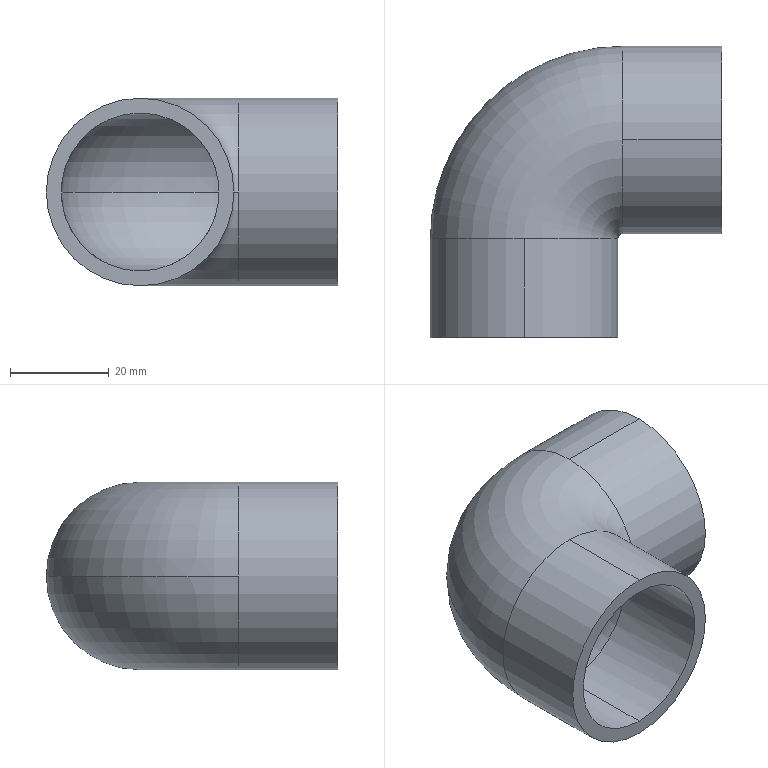Part | SolidWorks | features Sweep 1 | 1 solid | 14 faces | box 59 x 59 x 38 mm | volume 23558 mm3 | cylinder 8 | torus 4 | plane 2 | commonest cylinder face diameters 32 x4 38 x4
STEP:
#1=CARTESIAN_POINT('',(-16.,20.,0.));
#2=VERTEX_POINT('',#1);
#3=CARTESIAN_POINT('',(0.,20.,16.));
#4=VERTEX_POINT('',#3);
#5=CARTESIAN_POINT('',(0.,20.,0.));
#6=DIRECTION('',(0.,1.,0.));
#7=DIRECTION('',(0.,0.,1.));
#8=AXIS2_PLACEMENT_3D('',#5,#6,#7);
#9=CIRCLE('',#8,16.);
#10=EDGE_CURVE('',#2,#4,#9,.T.);
#11=ORIENTED_EDGE('',*,*,#10,.F.);
#12=CARTESIAN_POINT('',(20.,56.,0.));
#13=VERTEX_POINT('',#12);
#14=CARTESIAN_POINT('',(20.,20.,0.));
#15=DIRECTION('',(0.,0.,-1.));
#16=DIRECTION('',(-1.,0.,0.));
#17=AXIS2_PLACEMENT_3D('',#14,#15,#16);
#18=CIRCLE('',#17,36.);
#19=EDGE_CURVE('',#2,#13,#18,.T.);
#20=ORIENTED_EDGE('',*,*,#19,.T.);
#21=CARTESIAN_POINT('',(20.,40.,16.));
#22=VERTEX_POINT('',#21);
#23=CARTESIAN_POINT('',(20.,40.,0.));
#24=DIRECTION('',(1.,0.,0.));
#25=DIRECTION('',(0.,0.,1.));
#26=AXIS2_PLACEMENT_3D('',#23,#24,#25);
#27=CIRCLE('',#26,16.);
#28=EDGE_CURVE('',#13,#22,#27,.T.);
#29=ORIENTED_EDGE('',*,*,#28,.T.);
#30=CARTESIAN_POINT('',(20.,24.,0.));
#31=VERTEX_POINT('',#30);
#32=CARTESIAN_POINT('',(20.,40.,0.));
#33=DIRECTION('',(1.,0.,0.));
#34=DIRECTION('',(0.,0.,1.));
#35=AXIS2_PLACEMENT_3D('',#32,#33,#34);
#36=CIRCLE('',#35,16.);
#37=EDGE_CURVE('',#22,#31,#36,.T.);
#38=ORIENTED_EDGE('',*,*,#37,.T.);
#39=CARTESIAN_POINT('',(16.,20.,0.));
#40=VERTEX_POINT('',#39);
#41=CARTESIAN_POINT('',(20.,20.,0.));
#42=DIRECTION('',(0.,0.,-1.));
#43=DIRECTION('',(-1.,0.,0.));
#44=AXIS2_PLACEMENT_3D('',#41,#42,#43);
#45=CIRCLE('',#44,4.);
#46=EDGE_CURVE('',#40,#31,#45,.T.);
#47=ORIENTED_EDGE('',*,*,#46,.F.);
#48=CARTESIAN_POINT('',(0.,20.,0.));
#49=DIRECTION('',(0.,1.,0.));
#50=DIRECTION('',(0.,0.,1.));
#51=AXIS2_PLACEMENT_3D('',#48,#49,#50);
#52=CIRCLE('',#51,16.);
#53=EDGE_CURVE('',#4,#40,#52,.T.);
#54=ORIENTED_EDGE('',*,*,#53,.F.);
#55=EDGE_LOOP('',(#11,#20,#29,#38,#47,#54));
#56=FACE_OUTER_BOUND('',#55,.T.);
#57=CARTESIAN_POINT('',(20.,20.,0.));
#58=DIRECTION('',(0.,0.,-1.));
#59=DIRECTION('',(-1.,0.,0.));
#60=AXIS2_PLACEMENT_3D('',#57,#58,#59);
#61=TOROIDAL_SURFACE('',#60,20.,16.);
#62=ADVANCED_FACE('',(#56),#61,.F.);
#63=CARTESIAN_POINT('',(0.,20.,-19.));
#64=VERTEX_POINT('',#63);
#65=CARTESIAN_POINT('',(-19.,20.,0.));
#66=VERTEX_POINT('',#65);
#67=CARTESIAN_POINT('',(0.,20.,0.));
#68=DIRECTION('',(0.,1.,0.));
#69=DIRECTION('',(0.,0.,1.));
#70=AXIS2_PLACEMENT_3D('',#67,#68,#69);
#71=CIRCLE('',#70,19.);
#72=EDGE_CURVE('',#64,#66,#71,.T.);
#73=ORIENTED_EDGE('',*,*,#72,.T.);
#74=CARTESIAN_POINT('',(20.,59.,0.));
#75=VERTEX_POINT('',#74);
#76=CARTESIAN_POINT('',(20.,20.,0.));
#77=DIRECTION('',(0.,0.,-1.));
#78=DIRECTION('',(-1.,0.,0.));
#79=AXIS2_PLACEMENT_3D('',#76,#77,#78);
#80=CIRCLE('',#79,39.);
#81=EDGE_CURVE('',#66,#75,#80,.T.);
#82=ORIENTED_EDGE('',*,*,#81,.T.);
#83=CARTESIAN_POINT('',(20.,40.,-19.));
#84=VERTEX_POINT('',#83);
#85=CARTESIAN_POINT('',(20.,40.,0.));
#86=DIRECTION('',(1.,0.,0.));
#87=DIRECTION('',(0.,0.,1.));
#88=AXIS2_PLACEMENT_3D('',#85,#86,#87);
#89=CIRCLE('',#88,19.);
#90=EDGE_CURVE('',#84,#75,#89,.T.);
#91=ORIENTED_EDGE('',*,*,#90,.F.);
#92=CARTESIAN_POINT('',(20.,21.,0.));
#93=VERTEX_POINT('',#92);
#94=CARTESIAN_POINT('',(20.,40.,0.));
#95=DIRECTION('',(1.,0.,0.));
#96=DIRECTION('',(0.,0.,1.));
#97=AXIS2_PLACEMENT_3D('',#94,#95,#96);
#98=CIRCLE('',#97,19.);
#99=EDGE_CURVE('',#93,#84,#98,.T.);
#100=ORIENTED_EDGE('',*,*,#99,.F.);
#101=CARTESIAN_POINT('',(19.,20.,0.));
#102=VERTEX_POINT('',#101);
#103=CARTESIAN_POINT('',(20.,20.,0.));
#104=DIRECTION('',(0.,0.,-1.));
#105=DIRECTION('',(-1.,0.,0.));
#106=AXIS2_PLACEMENT_3D('',#103,#104,#105);
#107=CIRCLE('',#106,1.);
#108=EDGE_CURVE('',#102,#93,#107,.T.);
#109=ORIENTED_EDGE('',*,*,#108,.F.);
#110=CARTESIAN_POINT('',(0.,20.,0.));
#111=DIRECTION('',(0.,1.,0.));
#112=DIRECTION('',(0.,0.,1.));
#113=AXIS2_PLACEMENT_3D('',#110,#111,#112);
#114=CIRCLE('',#113,19.);
#115=EDGE_CURVE('',#102,#64,#114,.T.);
#116=ORIENTED_EDGE('',*,*,#115,.T.);
#117=EDGE_LOOP('',(#73,#82,#91,#100,#109,#116));
#118=FACE_OUTER_BOUND('',#117,.T.);
#119=CARTESIAN_POINT('',(20.,20.,0.));
#120=DIRECTION('',(0.,0.,-1.));
#121=DIRECTION('',(-1.,0.,0.));
#122=AXIS2_PLACEMENT_3D('',#119,#120,#121);
#123=TOROIDAL_SURFACE('',#122,20.,19.);
#124=ADVANCED_FACE('',(#118),#123,.T.);
#125=CARTESIAN_POINT('',(0.,20.,19.));
#126=VERTEX_POINT('',#125);
#127=CARTESIAN_POINT('',(0.,20.,0.));
#128=DIRECTION('',(0.,1.,0.));
#129=DIRECTION('',(0.,0.,1.));
#130=AXIS2_PLACEMENT_3D('',#127,#128,#129);
#131=CIRCLE('',#130,19.);
#132=EDGE_CURVE('',#126,#102,#131,.T.);
#133=ORIENTED_EDGE('',*,*,#132,.F.);
#134=CARTESIAN_POINT('',(0.,0.,19.));
#135=VERTEX_POINT('',#134);
#136=CARTESIAN_POINT('',(0.,20.,19.));
#137=DIRECTION('',(0.,-1.,0.));
#138=VECTOR('',#137,1000.);
#139=LINE('',#136,#138);
#140=EDGE_CURVE('',#126,#135,#139,.T.);
#141=ORIENTED_EDGE('',*,*,#140,.T.);
#142=CARTESIAN_POINT('',(0.,0.,-19.));
#143=VERTEX_POINT('',#142);
#144=CARTESIAN_POINT('',(0.,0.,0.));
#145=DIRECTION('',(0.,1.,0.));
#146=DIRECTION('',(0.,0.,1.));
#147=AXIS2_PLACEMENT_3D('',#144,#145,#146);
#148=CIRCLE('',#147,19.);
#149=EDGE_CURVE('',#135,#143,#148,.T.);
#150=ORIENTED_EDGE('',*,*,#149,.T.);
#151=CARTESIAN_POINT('',(0.,20.,-19.));
#152=DIRECTION('',(0.,-1.,0.));
#153=VECTOR('',#152,1000.);
#154=LINE('',#151,#153);
#155=EDGE_CURVE('',#64,#143,#154,.T.);
#156=ORIENTED_EDGE('',*,*,#155,.F.);
#157=ORIENTED_EDGE('',*,*,#115,.F.);
#158=EDGE_LOOP('',(#133,#141,#150,#156,#157));
#159=FACE_OUTER_BOUND('',#158,.T.);
#160=CARTESIAN_POINT('',(0.,20.,0.));
#161=DIRECTION('',(0.,-1.,0.));
#162=DIRECTION('',(0.,0.,-1.));
#163=AXIS2_PLACEMENT_3D('',#160,#161,#162);
#164=CYLINDRICAL_SURFACE('',#163,19.);
#165=ADVANCED_FACE('',(#159),#164,.T.);
#166=CARTESIAN_POINT('',(0.,20.,-16.));
#167=VERTEX_POINT('',#166);
#168=CARTESIAN_POINT('',(0.,20.,0.));
#169=DIRECTION('',(0.,1.,0.));
#170=DIRECTION('',(0.,0.,1.));
#171=AXIS2_PLACEMENT_3D('',#168,#169,#170);
#172=CIRCLE('',#171,16.);
#173=EDGE_CURVE('',#167,#2,#172,.T.);
#174=ORIENTED_EDGE('',*,*,#173,.T.);
#175=ORIENTED_EDGE('',*,*,#10,.T.);
#176=CARTESIAN_POINT('',(0.,0.,16.));
#177=VERTEX_POINT('',#176);
#178=CARTESIAN_POINT('',(0.,20.,16.));
#179=DIRECTION('',(0.,-1.,0.));
#180=VECTOR('',#179,1000.);
#181=LINE('',#178,#180);
#182=EDGE_CURVE('',#4,#177,#181,.T.);
#183=ORIENTED_EDGE('',*,*,#182,.T.);
#184=CARTESIAN_POINT('',(0.,0.,-16.));
#185=VERTEX_POINT('',#184);
#186=CARTESIAN_POINT('',(0.,0.,0.));
#187=DIRECTION('',(0.,1.,0.));
#188=DIRECTION('',(0.,0.,1.));
#189=AXIS2_PLACEMENT_3D('',#186,#187,#188);
#190=CIRCLE('',#189,16.);
#191=EDGE_CURVE('',#185,#177,#190,.T.);
#192=ORIENTED_EDGE('',*,*,#191,.F.);
#193=CARTESIAN_POINT('',(0.,20.,-16.));
#194=DIRECTION('',(0.,-1.,0.));
#195=VECTOR('',#194,1000.);
#196=LINE('',#193,#195);
#197=EDGE_CURVE('',#167,#185,#196,.T.);
#198=ORIENTED_EDGE('',*,*,#197,.F.);
#199=EDGE_LOOP('',(#174,#175,#183,#192,#198));
#200=FACE_OUTER_BOUND('',#199,.T.);
#201=CARTESIAN_POINT('',(0.,20.,0.));
#202=DIRECTION('',(0.,-1.,0.));
#203=DIRECTION('',(0.,0.,-1.));
#204=AXIS2_PLACEMENT_3D('',#201,#202,#203);
#205=CYLINDRICAL_SURFACE('',#204,16.);
#206=ADVANCED_FACE('',(#200),#205,.F.);
#207=ORIENTED_EDGE('',*,*,#37,.F.);
#208=CARTESIAN_POINT('',(40.,40.,16.));
#209=VERTEX_POINT('',#208);
#210=CARTESIAN_POINT('',(20.,40.,16.));
#211=DIRECTION('',(1.,0.,0.));
#212=VECTOR('',#211,1000.);
#213=LINE('',#210,#212);
#214=EDGE_CURVE('',#22,#209,#213,.T.);
#215=ORIENTED_EDGE('',*,*,#214,.T.);
#216=CARTESIAN_POINT('',(40.,40.,-16.));
#217=VERTEX_POINT('',#216);
#218=CARTESIAN_POINT('',(40.,40.,0.));
#219=DIRECTION('',(1.,0.,0.));
#220=DIRECTION('',(0.,0.,1.));
#221=AXIS2_PLACEMENT_3D('',#218,#219,#220);
#222=CIRCLE('',#221,16.);
#223=EDGE_CURVE('',#209,#217,#222,.T.);
#224=ORIENTED_EDGE('',*,*,#223,.T.);
#225=CARTESIAN_POINT('',(20.,40.,-16.));
#226=VERTEX_POINT('',#225);
#227=CARTESIAN_POINT('',(20.,40.,-16.));
#228=DIRECTION('',(1.,0.,0.));
#229=VECTOR('',#228,1000.);
#230=LINE('',#227,#229);
#231=EDGE_CURVE('',#226,#217,#230,.T.);
#232=ORIENTED_EDGE('',*,*,#231,.F.);
#233=CARTESIAN_POINT('',(20.,40.,0.));
#234=DIRECTION('',(1.,0.,0.));
#235=DIRECTION('',(0.,0.,1.));
#236=AXIS2_PLACEMENT_3D('',#233,#234,#235);
#237=CIRCLE('',#236,16.);
#238=EDGE_CURVE('',#31,#226,#237,.T.);
#239=ORIENTED_EDGE('',*,*,#238,.F.);
#240=EDGE_LOOP('',(#207,#215,#224,#232,#239));
#241=FACE_OUTER_BOUND('',#240,.T.);
#242=CARTESIAN_POINT('',(20.,40.,0.));
#243=DIRECTION('',(1.,0.,0.));
#244=DIRECTION('',(0.,0.,-1.));
#245=AXIS2_PLACEMENT_3D('',#242,#243,#244);
#246=CYLINDRICAL_SURFACE('',#245,16.);
#247=ADVANCED_FACE('',(#241),#246,.F.);
#248=ORIENTED_EDGE('',*,*,#90,.T.);
#249=CARTESIAN_POINT('',(20.,40.,19.));
#250=VERTEX_POINT('',#249);
#251=CARTESIAN_POINT('',(20.,40.,0.));
#252=DIRECTION('',(1.,0.,0.));
#253=DIRECTION('',(0.,0.,1.));
#254=AXIS2_PLACEMENT_3D('',#251,#252,#253);
#255=CIRCLE('',#254,19.);
#256=EDGE_CURVE('',#75,#250,#255,.T.);
#257=ORIENTED_EDGE('',*,*,#256,.T.);
#258=CARTESIAN_POINT('',(40.,40.,19.));
#259=VERTEX_POINT('',#258);
#260=CARTESIAN_POINT('',(20.,40.,19.));
#261=DIRECTION('',(1.,0.,0.));
#262=VECTOR('',#261,1000.);
#263=LINE('',#260,#262);
#264=EDGE_CURVE('',#250,#259,#263,.T.);
#265=ORIENTED_EDGE('',*,*,#264,.T.);
#266=CARTESIAN_POINT('',(40.,40.,-19.));
#267=VERTEX_POINT('',#266);
#268=CARTESIAN_POINT('',(40.,40.,0.));
#269=DIRECTION('',(1.,0.,0.));
#270=DIRECTION('',(0.,0.,1.));
#271=AXIS2_PLACEMENT_3D('',#268,#269,#270);
#272=CIRCLE('',#271,19.);
#273=EDGE_CURVE('',#267,#259,#272,.T.);
#274=ORIENTED_EDGE('',*,*,#273,.F.);
#275=CARTESIAN_POINT('',(20.,40.,-19.));
#276=DIRECTION('',(1.,0.,0.));
#277=VECTOR('',#276,1000.);
#278=LINE('',#275,#277);
#279=EDGE_CURVE('',#84,#267,#278,.T.);
#280=ORIENTED_EDGE('',*,*,#279,.F.);
#281=EDGE_LOOP('',(#248,#257,#265,#274,#280));
#282=FACE_OUTER_BOUND('',#281,.T.);
#283=CARTESIAN_POINT('',(20.,40.,0.));
#284=DIRECTION('',(1.,0.,0.));
#285=DIRECTION('',(0.,0.,-1.));
#286=AXIS2_PLACEMENT_3D('',#283,#284,#285);
#287=CYLINDRICAL_SURFACE('',#286,19.);
#288=ADVANCED_FACE('',(#282),#287,.T.);
#289=ORIENTED_EDGE('',*,*,#264,.F.);
#290=CARTESIAN_POINT('',(20.,40.,0.));
#291=DIRECTION('',(1.,0.,0.));
#292=DIRECTION('',(0.,0.,1.));
#293=AXIS2_PLACEMENT_3D('',#290,#291,#292);
#294=CIRCLE('',#293,19.);
#295=EDGE_CURVE('',#250,#93,#294,.T.);
#296=ORIENTED_EDGE('',*,*,#295,.T.);
#297=ORIENTED_EDGE('',*,*,#99,.T.);
#298=ORIENTED_EDGE('',*,*,#279,.T.);
#299=CARTESIAN_POINT('',(40.,40.,0.));
#300=DIRECTION('',(1.,0.,0.));
#301=DIRECTION('',(0.,0.,1.));
#302=AXIS2_PLACEMENT_3D('',#299,#300,#301);
#303=CIRCLE('',#302,19.);
#304=EDGE_CURVE('',#259,#267,#303,.T.);
#305=ORIENTED_EDGE('',*,*,#304,.F.);
#306=EDGE_LOOP('',(#289,#296,#297,#298,#305));
#307=FACE_OUTER_BOUND('',#306,.T.);
#308=CARTESIAN_POINT('',(20.,40.,0.));
#309=DIRECTION('',(1.,0.,0.));
#310=DIRECTION('',(0.,0.,-1.));
#311=AXIS2_PLACEMENT_3D('',#308,#309,#310);
#312=CYLINDRICAL_SURFACE('',#311,19.);
#313=ADVANCED_FACE('',(#307),#312,.T.);
#314=ORIENTED_EDGE('',*,*,#214,.F.);
#315=ORIENTED_EDGE('',*,*,#28,.F.);
#316=CARTESIAN_POINT('',(20.,40.,0.));
#317=DIRECTION('',(1.,0.,0.));
#318=DIRECTION('',(0.,0.,1.));
#319=AXIS2_PLACEMENT_3D('',#316,#317,#318);
#320=CIRCLE('',#319,16.);
#321=EDGE_CURVE('',#226,#13,#320,.T.);
#322=ORIENTED_EDGE('',*,*,#321,.F.);
#323=ORIENTED_EDGE('',*,*,#231,.T.);
#324=CARTESIAN_POINT('',(40.,40.,0.));
#325=DIRECTION('',(1.,0.,0.));
#326=DIRECTION('',(0.,0.,1.));
#327=AXIS2_PLACEMENT_3D('',#324,#325,#326);
#328=CIRCLE('',#327,16.);
#329=EDGE_CURVE('',#217,#209,#328,.T.);
#330=ORIENTED_EDGE('',*,*,#329,.T.);
#331=EDGE_LOOP('',(#314,#315,#322,#323,#330));
#332=FACE_OUTER_BOUND('',#331,.T.);
#333=CARTESIAN_POINT('',(20.,40.,0.));
#334=DIRECTION('',(1.,0.,0.));
#335=DIRECTION('',(0.,0.,-1.));
#336=AXIS2_PLACEMENT_3D('',#333,#334,#335);
#337=CYLINDRICAL_SURFACE('',#336,16.);
#338=ADVANCED_FACE('',(#332),#337,.F.);
#339=ORIENTED_EDGE('',*,*,#81,.F.);
#340=CARTESIAN_POINT('',(0.,20.,0.));
#341=DIRECTION('',(0.,1.,0.));
#342=DIRECTION('',(0.,0.,1.));
#343=AXIS2_PLACEMENT_3D('',#340,#341,#342);
#344=CIRCLE('',#343,19.);
#345=EDGE_CURVE('',#66,#126,#344,.T.);
#346=ORIENTED_EDGE('',*,*,#345,.T.);
#347=ORIENTED_EDGE('',*,*,#132,.T.);
#348=ORIENTED_EDGE('',*,*,#108,.T.);
#349=ORIENTED_EDGE('',*,*,#295,.F.);
#350=ORIENTED_EDGE('',*,*,#256,.F.);
#351=EDGE_LOOP('',(#339,#346,#347,#348,#349,#350));
#352=FACE_OUTER_BOUND('',#351,.T.);
#353=CARTESIAN_POINT('',(20.,20.,0.));
#354=DIRECTION('',(0.,0.,-1.));
#355=DIRECTION('',(-1.,0.,0.));
#356=AXIS2_PLACEMENT_3D('',#353,#354,#355);
#357=TOROIDAL_SURFACE('',#356,20.,19.);
#358=ADVANCED_FACE('',(#352),#357,.T.);
#359=ORIENTED_EDGE('',*,*,#19,.F.);
#360=ORIENTED_EDGE('',*,*,#173,.F.);
#361=CARTESIAN_POINT('',(0.,20.,0.));
#362=DIRECTION('',(0.,1.,0.));
#363=DIRECTION('',(0.,0.,1.));
#364=AXIS2_PLACEMENT_3D('',#361,#362,#363);
#365=CIRCLE('',#364,16.);
#366=EDGE_CURVE('',#40,#167,#365,.T.);
#367=ORIENTED_EDGE('',*,*,#366,.F.);
#368=ORIENTED_EDGE('',*,*,#46,.T.);
#369=ORIENTED_EDGE('',*,*,#238,.T.);
#370=ORIENTED_EDGE('',*,*,#321,.T.);
#371=EDGE_LOOP('',(#359,#360,#367,#368,#369,#370));
#372=FACE_OUTER_BOUND('',#371,.T.);
#373=CARTESIAN_POINT('',(20.,20.,0.));
#374=DIRECTION('',(0.,0.,-1.));
#375=DIRECTION('',(-1.,0.,0.));
#376=AXIS2_PLACEMENT_3D('',#373,#374,#375);
#377=TOROIDAL_SURFACE('',#376,20.,16.);
#378=ADVANCED_FACE('',(#372),#377,.F.);
#379=ORIENTED_EDGE('',*,*,#182,.F.);
#380=ORIENTED_EDGE('',*,*,#53,.T.);
#381=ORIENTED_EDGE('',*,*,#366,.T.);
#382=ORIENTED_EDGE('',*,*,#197,.T.);
#383=CARTESIAN_POINT('',(0.,0.,0.));
#384=DIRECTION('',(0.,1.,0.));
#385=DIRECTION('',(0.,0.,1.));
#386=AXIS2_PLACEMENT_3D('',#383,#384,#385);
#387=CIRCLE('',#386,16.);
#388=EDGE_CURVE('',#177,#185,#387,.T.);
#389=ORIENTED_EDGE('',*,*,#388,.F.);
#390=EDGE_LOOP('',(#379,#380,#381,#382,#389));
#391=FACE_OUTER_BOUND('',#390,.T.);
#392=CARTESIAN_POINT('',(0.,20.,0.));
#393=DIRECTION('',(0.,-1.,0.));
#394=DIRECTION('',(0.,0.,-1.));
#395=AXIS2_PLACEMENT_3D('',#392,#393,#394);
#396=CYLINDRICAL_SURFACE('',#395,16.);
#397=ADVANCED_FACE('',(#391),#396,.F.);
#398=ORIENTED_EDGE('',*,*,#140,.F.);
#399=ORIENTED_EDGE('',*,*,#345,.F.);
#400=ORIENTED_EDGE('',*,*,#72,.F.);
#401=ORIENTED_EDGE('',*,*,#155,.T.);
#402=CARTESIAN_POINT('',(0.,0.,0.));
#403=DIRECTION('',(0.,1.,0.));
#404=DIRECTION('',(0.,0.,1.));
#405=AXIS2_PLACEMENT_3D('',#402,#403,#404);
#406=CIRCLE('',#405,19.);
#407=EDGE_CURVE('',#143,#135,#406,.T.);
#408=ORIENTED_EDGE('',*,*,#407,.T.);
#409=EDGE_LOOP('',(#398,#399,#400,#401,#408));
#410=FACE_OUTER_BOUND('',#409,.T.);
#411=CARTESIAN_POINT('',(0.,20.,0.));
#412=DIRECTION('',(0.,-1.,0.));
#413=DIRECTION('',(0.,0.,-1.));
#414=AXIS2_PLACEMENT_3D('',#411,#412,#413);
#415=CYLINDRICAL_SURFACE('',#414,19.);
#416=ADVANCED_FACE('',(#410),#415,.T.);
#417=ORIENTED_EDGE('',*,*,#329,.F.);
#418=ORIENTED_EDGE('',*,*,#223,.F.);
#419=EDGE_LOOP('',(#417,#418));
#420=FACE_BOUND('',#419,.T.);
#421=ORIENTED_EDGE('',*,*,#273,.T.);
#422=ORIENTED_EDGE('',*,*,#304,.T.);
#423=EDGE_LOOP('',(#421,#422));
#424=FACE_OUTER_BOUND('',#423,.T.);
#425=CARTESIAN_POINT('',(40.,40.,0.));
#426=DIRECTION('',(1.,0.,0.));
#427=DIRECTION('',(0.,0.,1.));
#428=AXIS2_PLACEMENT_3D('',#425,#426,#427);
#429=PLANE('',#428);
#430=ADVANCED_FACE('',(#420,#424),#429,.T.);
#431=ORIENTED_EDGE('',*,*,#191,.T.);
#432=ORIENTED_EDGE('',*,*,#388,.T.);
#433=EDGE_LOOP('',(#431,#432));
#434=FACE_BOUND('',#433,.T.);
#435=ORIENTED_EDGE('',*,*,#407,.F.);
#436=ORIENTED_EDGE('',*,*,#149,.F.);
#437=EDGE_LOOP('',(#435,#436));
#438=FACE_OUTER_BOUND('',#437,.T.);
#439=CARTESIAN_POINT('',(0.,0.,0.));
#440=DIRECTION('',(0.,1.,0.));
#441=DIRECTION('',(0.,0.,1.));
#442=AXIS2_PLACEMENT_3D('',#439,#440,#441);
#443=PLANE('',#442);
#444=ADVANCED_FACE('',(#434,#438),#443,.F.);
#445=CLOSED_SHELL('',(#62,#124,#165,#206,#247,#288,#313,#338,#358,#378,#397,#416,#430,#444));
#446=MANIFOLD_SOLID_BREP('',#445);
#447=CARTESIAN_POINT('',(0.,0.,0.));
#448=DIRECTION('',(0.,0.,1.));
#449=DIRECTION('',(1.,0.,0.));
#450=AXIS2_PLACEMENT_3D('',#447,#448,#449);
#451=(LENGTH_UNIT()NAMED_UNIT(*)SI_UNIT(.MILLI.,.METRE.));
#452=UNCERTAINTY_MEASURE_WITH_UNIT(LENGTH_MEASURE(0.00001),#451,'','');
#453=(NAMED_UNIT(*)PLANE_ANGLE_UNIT()SI_UNIT($,.RADIAN.));
#454=(NAMED_UNIT(*)SI_UNIT($,.STERADIAN.)SOLID_ANGLE_UNIT());
#455=(GEOMETRIC_REPRESENTATION_CONTEXT(3)GLOBAL_UNCERTAINTY_ASSIGNED_CONTEXT((#452))GLOBAL_UNIT_ASSIGNED_CONTEXT((#451,#453,#454))REPRESENTATION_CONTEXT('',''));
#456=ADVANCED_BREP_SHAPE_REPRESENTATION('',(#446,#450),#455);